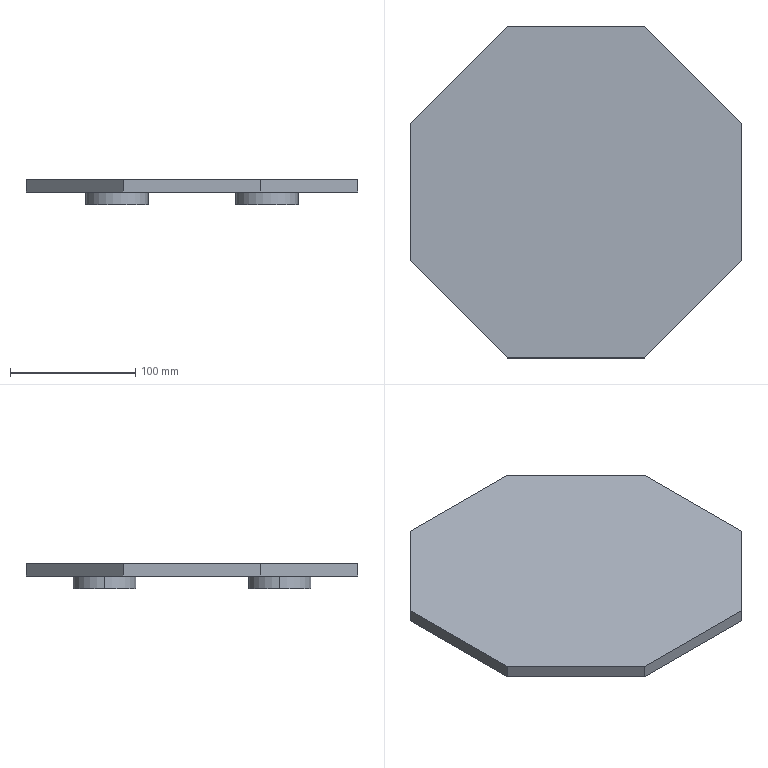Part | SolidWorks | features Extrusion 1, ICE 1 | 1 solid | 28 faces | box 265.563 x 265.563 x 20 mm | volume 605445 mm3 | plane 16 | cylinder 12 | commonest cylinder face diameters 40 x6 50 x6
STEP:
#1=CARTESIAN_POINT('',(-559.884,-160.,-10.));
#2=VERTEX_POINT('',#1);
#3=CARTESIAN_POINT('',(-519.884,-160.,-10.));
#4=VERTEX_POINT('',#3);
#5=CARTESIAN_POINT('',(-539.884,-160.,-10.));
#6=DIRECTION('',(0.,0.,1.));
#7=DIRECTION('',(1.,0.,0.));
#8=AXIS2_PLACEMENT_3D('',#5,#6,#7);
#9=CIRCLE('',#8,20.);
#10=EDGE_CURVE('',#2,#4,#9,.T.);
#11=ORIENTED_EDGE('',*,*,#10,.F.);
#12=CARTESIAN_POINT('',(-559.884,-160.,0.));
#13=VERTEX_POINT('',#12);
#14=CARTESIAN_POINT('',(-559.884,-160.,-10.));
#15=DIRECTION('',(0.,0.,1.));
#16=VECTOR('',#15,1000.);
#17=LINE('',#14,#16);
#18=EDGE_CURVE('',#2,#13,#17,.T.);
#19=ORIENTED_EDGE('',*,*,#18,.T.);
#20=CARTESIAN_POINT('',(-519.884,-160.,0.));
#21=VERTEX_POINT('',#20);
#22=CARTESIAN_POINT('',(-539.884,-160.,0.));
#23=DIRECTION('',(0.,0.,1.));
#24=DIRECTION('',(1.,0.,0.));
#25=AXIS2_PLACEMENT_3D('',#22,#23,#24);
#26=CIRCLE('',#25,20.);
#27=EDGE_CURVE('',#13,#21,#26,.T.);
#28=ORIENTED_EDGE('',*,*,#27,.T.);
#29=CARTESIAN_POINT('',(-519.884,-160.,-10.));
#30=DIRECTION('',(0.,0.,1.));
#31=VECTOR('',#30,1000.);
#32=LINE('',#29,#31);
#33=EDGE_CURVE('',#4,#21,#32,.T.);
#34=ORIENTED_EDGE('',*,*,#33,.F.);
#35=EDGE_LOOP('',(#11,#19,#28,#34));
#36=FACE_OUTER_BOUND('',#35,.T.);
#37=CARTESIAN_POINT('',(-539.884,-160.,-10.));
#38=DIRECTION('',(0.,0.,1.));
#39=DIRECTION('',(1.,0.,0.));
#40=AXIS2_PLACEMENT_3D('',#37,#38,#39);
#41=CYLINDRICAL_SURFACE('',#40,20.);
#42=ADVANCED_FACE('',(#36),#41,.F.);
#43=CARTESIAN_POINT('',(-514.884,-160.,-10.));
#44=VERTEX_POINT('',#43);
#45=CARTESIAN_POINT('',(-564.884,-160.,-10.));
#46=VERTEX_POINT('',#45);
#47=CARTESIAN_POINT('',(-539.884,-160.,-10.));
#48=DIRECTION('',(0.,0.,1.));
#49=DIRECTION('',(1.,0.,0.));
#50=AXIS2_PLACEMENT_3D('',#47,#48,#49);
#51=CIRCLE('',#50,25.);
#52=EDGE_CURVE('',#44,#46,#51,.T.);
#53=ORIENTED_EDGE('',*,*,#52,.T.);
#54=CARTESIAN_POINT('',(-564.884,-160.,0.));
#55=VERTEX_POINT('',#54);
#56=CARTESIAN_POINT('',(-564.884,-160.,-10.));
#57=DIRECTION('',(0.,0.,1.));
#58=VECTOR('',#57,1000.);
#59=LINE('',#56,#58);
#60=EDGE_CURVE('',#46,#55,#59,.T.);
#61=ORIENTED_EDGE('',*,*,#60,.T.);
#62=CARTESIAN_POINT('',(-514.884,-160.,0.));
#63=VERTEX_POINT('',#62);
#64=CARTESIAN_POINT('',(-539.884,-160.,0.));
#65=DIRECTION('',(0.,0.,1.));
#66=DIRECTION('',(1.,0.,0.));
#67=AXIS2_PLACEMENT_3D('',#64,#65,#66);
#68=CIRCLE('',#67,25.);
#69=EDGE_CURVE('',#63,#55,#68,.T.);
#70=ORIENTED_EDGE('',*,*,#69,.F.);
#71=CARTESIAN_POINT('',(-514.884,-160.,-10.));
#72=DIRECTION('',(0.,0.,1.));
#73=VECTOR('',#72,1000.);
#74=LINE('',#71,#73);
#75=EDGE_CURVE('',#44,#63,#74,.T.);
#76=ORIENTED_EDGE('',*,*,#75,.F.);
#77=EDGE_LOOP('',(#53,#61,#70,#76));
#78=FACE_OUTER_BOUND('',#77,.T.);
#79=CARTESIAN_POINT('',(-539.884,-160.,-10.));
#80=DIRECTION('',(0.,0.,1.));
#81=DIRECTION('',(1.,0.,0.));
#82=AXIS2_PLACEMENT_3D('',#79,#80,#81);
#83=CYLINDRICAL_SURFACE('',#82,25.);
#84=ADVANCED_FACE('',(#78),#83,.T.);
#85=CARTESIAN_POINT('',(-559.884,-20.,-10.));
#86=VERTEX_POINT('',#85);
#87=CARTESIAN_POINT('',(-519.884,-20.,-10.));
#88=VERTEX_POINT('',#87);
#89=CARTESIAN_POINT('',(-539.884,-20.,-10.));
#90=DIRECTION('',(0.,0.,1.));
#91=DIRECTION('',(1.,0.,0.));
#92=AXIS2_PLACEMENT_3D('',#89,#90,#91);
#93=CIRCLE('',#92,20.);
#94=EDGE_CURVE('',#86,#88,#93,.T.);
#95=ORIENTED_EDGE('',*,*,#94,.F.);
#96=CARTESIAN_POINT('',(-559.884,-20.,0.));
#97=VERTEX_POINT('',#96);
#98=CARTESIAN_POINT('',(-559.884,-20.,-10.));
#99=DIRECTION('',(0.,0.,1.));
#100=VECTOR('',#99,1000.);
#101=LINE('',#98,#100);
#102=EDGE_CURVE('',#86,#97,#101,.T.);
#103=ORIENTED_EDGE('',*,*,#102,.T.);
#104=CARTESIAN_POINT('',(-519.884,-20.,0.));
#105=VERTEX_POINT('',#104);
#106=CARTESIAN_POINT('',(-539.884,-20.,0.));
#107=DIRECTION('',(0.,0.,1.));
#108=DIRECTION('',(1.,0.,0.));
#109=AXIS2_PLACEMENT_3D('',#106,#107,#108);
#110=CIRCLE('',#109,20.);
#111=EDGE_CURVE('',#97,#105,#110,.T.);
#112=ORIENTED_EDGE('',*,*,#111,.T.);
#113=CARTESIAN_POINT('',(-519.884,-20.,-10.));
#114=DIRECTION('',(0.,0.,1.));
#115=VECTOR('',#114,1000.);
#116=LINE('',#113,#115);
#117=EDGE_CURVE('',#88,#105,#116,.T.);
#118=ORIENTED_EDGE('',*,*,#117,.F.);
#119=EDGE_LOOP('',(#95,#103,#112,#118));
#120=FACE_OUTER_BOUND('',#119,.T.);
#121=CARTESIAN_POINT('',(-539.884,-20.,-10.));
#122=DIRECTION('',(0.,0.,1.));
#123=DIRECTION('',(1.,0.,0.));
#124=AXIS2_PLACEMENT_3D('',#121,#122,#123);
#125=CYLINDRICAL_SURFACE('',#124,20.);
#126=ADVANCED_FACE('',(#120),#125,.F.);
#127=CARTESIAN_POINT('',(-514.884,-20.,-10.));
#128=VERTEX_POINT('',#127);
#129=CARTESIAN_POINT('',(-564.884,-20.,-10.));
#130=VERTEX_POINT('',#129);
#131=CARTESIAN_POINT('',(-539.884,-20.,-10.));
#132=DIRECTION('',(0.,0.,1.));
#133=DIRECTION('',(1.,0.,0.));
#134=AXIS2_PLACEMENT_3D('',#131,#132,#133);
#135=CIRCLE('',#134,25.);
#136=EDGE_CURVE('',#128,#130,#135,.T.);
#137=ORIENTED_EDGE('',*,*,#136,.T.);
#138=CARTESIAN_POINT('',(-564.884,-20.,0.));
#139=VERTEX_POINT('',#138);
#140=CARTESIAN_POINT('',(-564.884,-20.,-10.));
#141=DIRECTION('',(0.,0.,1.));
#142=VECTOR('',#141,1000.);
#143=LINE('',#140,#142);
#144=EDGE_CURVE('',#130,#139,#143,.T.);
#145=ORIENTED_EDGE('',*,*,#144,.T.);
#146=CARTESIAN_POINT('',(-514.884,-20.,0.));
#147=VERTEX_POINT('',#146);
#148=CARTESIAN_POINT('',(-539.884,-20.,0.));
#149=DIRECTION('',(0.,0.,1.));
#150=DIRECTION('',(1.,0.,0.));
#151=AXIS2_PLACEMENT_3D('',#148,#149,#150);
#152=CIRCLE('',#151,25.);
#153=EDGE_CURVE('',#147,#139,#152,.T.);
#154=ORIENTED_EDGE('',*,*,#153,.F.);
#155=CARTESIAN_POINT('',(-514.884,-20.,-10.));
#156=DIRECTION('',(0.,0.,1.));
#157=VECTOR('',#156,1000.);
#158=LINE('',#155,#157);
#159=EDGE_CURVE('',#128,#147,#158,.T.);
#160=ORIENTED_EDGE('',*,*,#159,.F.);
#161=EDGE_LOOP('',(#137,#145,#154,#160));
#162=FACE_OUTER_BOUND('',#161,.T.);
#163=CARTESIAN_POINT('',(-539.884,-20.,-10.));
#164=DIRECTION('',(0.,0.,1.));
#165=DIRECTION('',(1.,0.,0.));
#166=AXIS2_PLACEMENT_3D('',#163,#164,#165);
#167=CYLINDRICAL_SURFACE('',#166,25.);
#168=ADVANCED_FACE('',(#162),#167,.T.);
#169=CARTESIAN_POINT('',(-679.884,-20.,-10.));
#170=VERTEX_POINT('',#169);
#171=CARTESIAN_POINT('',(-639.884,-20.,-10.));
#172=VERTEX_POINT('',#171);
#173=CARTESIAN_POINT('',(-659.884,-20.,-10.));
#174=DIRECTION('',(0.,0.,1.));
#175=DIRECTION('',(1.,0.,0.));
#176=AXIS2_PLACEMENT_3D('',#173,#174,#175);
#177=CIRCLE('',#176,20.);
#178=EDGE_CURVE('',#170,#172,#177,.T.);
#179=ORIENTED_EDGE('',*,*,#178,.F.);
#180=CARTESIAN_POINT('',(-679.884,-20.,0.));
#181=VERTEX_POINT('',#180);
#182=CARTESIAN_POINT('',(-679.884,-20.,-10.));
#183=DIRECTION('',(0.,0.,1.));
#184=VECTOR('',#183,1000.);
#185=LINE('',#182,#184);
#186=EDGE_CURVE('',#170,#181,#185,.T.);
#187=ORIENTED_EDGE('',*,*,#186,.T.);
#188=CARTESIAN_POINT('',(-639.884,-20.,0.));
#189=VERTEX_POINT('',#188);
#190=CARTESIAN_POINT('',(-659.884,-20.,0.));
#191=DIRECTION('',(0.,0.,1.));
#192=DIRECTION('',(1.,0.,0.));
#193=AXIS2_PLACEMENT_3D('',#190,#191,#192);
#194=CIRCLE('',#193,20.);
#195=EDGE_CURVE('',#181,#189,#194,.T.);
#196=ORIENTED_EDGE('',*,*,#195,.T.);
#197=CARTESIAN_POINT('',(-639.884,-20.,-10.));
#198=DIRECTION('',(0.,0.,1.));
#199=VECTOR('',#198,1000.);
#200=LINE('',#197,#199);
#201=EDGE_CURVE('',#172,#189,#200,.T.);
#202=ORIENTED_EDGE('',*,*,#201,.F.);
#203=EDGE_LOOP('',(#179,#187,#196,#202));
#204=FACE_OUTER_BOUND('',#203,.T.);
#205=CARTESIAN_POINT('',(-659.884,-20.,-10.));
#206=DIRECTION('',(0.,0.,1.));
#207=DIRECTION('',(1.,0.,0.));
#208=AXIS2_PLACEMENT_3D('',#205,#206,#207);
#209=CYLINDRICAL_SURFACE('',#208,20.);
#210=ADVANCED_FACE('',(#204),#209,.F.);
#211=CARTESIAN_POINT('',(-634.884,-20.,-10.));
#212=VERTEX_POINT('',#211);
#213=CARTESIAN_POINT('',(-684.884,-20.,-10.));
#214=VERTEX_POINT('',#213);
#215=CARTESIAN_POINT('',(-659.884,-20.,-10.));
#216=DIRECTION('',(0.,0.,1.));
#217=DIRECTION('',(1.,0.,0.));
#218=AXIS2_PLACEMENT_3D('',#215,#216,#217);
#219=CIRCLE('',#218,25.);
#220=EDGE_CURVE('',#212,#214,#219,.T.);
#221=ORIENTED_EDGE('',*,*,#220,.T.);
#222=CARTESIAN_POINT('',(-684.884,-20.,0.));
#223=VERTEX_POINT('',#222);
#224=CARTESIAN_POINT('',(-684.884,-20.,-10.));
#225=DIRECTION('',(0.,0.,1.));
#226=VECTOR('',#225,1000.);
#227=LINE('',#224,#226);
#228=EDGE_CURVE('',#214,#223,#227,.T.);
#229=ORIENTED_EDGE('',*,*,#228,.T.);
#230=CARTESIAN_POINT('',(-634.884,-20.,0.));
#231=VERTEX_POINT('',#230);
#232=CARTESIAN_POINT('',(-659.884,-20.,0.));
#233=DIRECTION('',(0.,0.,1.));
#234=DIRECTION('',(1.,0.,0.));
#235=AXIS2_PLACEMENT_3D('',#232,#233,#234);
#236=CIRCLE('',#235,25.);
#237=EDGE_CURVE('',#231,#223,#236,.T.);
#238=ORIENTED_EDGE('',*,*,#237,.F.);
#239=CARTESIAN_POINT('',(-634.884,-20.,-10.));
#240=DIRECTION('',(0.,0.,1.));
#241=VECTOR('',#240,1000.);
#242=LINE('',#239,#241);
#243=EDGE_CURVE('',#212,#231,#242,.T.);
#244=ORIENTED_EDGE('',*,*,#243,.F.);
#245=EDGE_LOOP('',(#221,#229,#238,#244));
#246=FACE_OUTER_BOUND('',#245,.T.);
#247=CARTESIAN_POINT('',(-659.884,-20.,-10.));
#248=DIRECTION('',(0.,0.,1.));
#249=DIRECTION('',(1.,0.,0.));
#250=AXIS2_PLACEMENT_3D('',#247,#248,#249);
#251=CYLINDRICAL_SURFACE('',#250,25.);
#252=ADVANCED_FACE('',(#246),#251,.T.);
#253=ORIENTED_EDGE('',*,*,#228,.F.);
#254=CARTESIAN_POINT('',(-659.884,-20.,-10.));
#255=DIRECTION('',(0.,0.,1.));
#256=DIRECTION('',(1.,0.,0.));
#257=AXIS2_PLACEMENT_3D('',#254,#255,#256);
#258=CIRCLE('',#257,25.);
#259=EDGE_CURVE('',#214,#212,#258,.T.);
#260=ORIENTED_EDGE('',*,*,#259,.T.);
#261=ORIENTED_EDGE('',*,*,#243,.T.);
#262=CARTESIAN_POINT('',(-659.884,-20.,0.));
#263=DIRECTION('',(0.,0.,1.));
#264=DIRECTION('',(1.,0.,0.));
#265=AXIS2_PLACEMENT_3D('',#262,#263,#264);
#266=CIRCLE('',#265,25.);
#267=EDGE_CURVE('',#223,#231,#266,.T.);
#268=ORIENTED_EDGE('',*,*,#267,.F.);
#269=EDGE_LOOP('',(#253,#260,#261,#268));
#270=FACE_OUTER_BOUND('',#269,.T.);
#271=CARTESIAN_POINT('',(-659.884,-20.,-10.));
#272=DIRECTION('',(0.,0.,1.));
#273=DIRECTION('',(1.,0.,0.));
#274=AXIS2_PLACEMENT_3D('',#271,#272,#273);
#275=CYLINDRICAL_SURFACE('',#274,25.);
#276=ADVANCED_FACE('',(#270),#275,.T.);
#277=CARTESIAN_POINT('',(-659.884,-20.,-10.));
#278=DIRECTION('',(0.,0.,1.));
#279=DIRECTION('',(1.,0.,0.));
#280=AXIS2_PLACEMENT_3D('',#277,#278,#279);
#281=CIRCLE('',#280,20.);
#282=EDGE_CURVE('',#172,#170,#281,.T.);
#283=ORIENTED_EDGE('',*,*,#282,.T.);
#284=ORIENTED_EDGE('',*,*,#178,.T.);
#285=EDGE_LOOP('',(#283,#284));
#286=FACE_BOUND('',#285,.T.);
#287=ORIENTED_EDGE('',*,*,#220,.F.);
#288=ORIENTED_EDGE('',*,*,#259,.F.);
#289=EDGE_LOOP('',(#287,#288));
#290=FACE_OUTER_BOUND('',#289,.T.);
#291=CARTESIAN_POINT('',(-659.884,-20.,-10.));
#292=DIRECTION('',(0.,0.,1.));
#293=DIRECTION('',(1.,0.,0.));
#294=AXIS2_PLACEMENT_3D('',#291,#292,#293);
#295=PLANE('',#294);
#296=ADVANCED_FACE('',(#286,#290),#295,.F.);
#297=ORIENTED_EDGE('',*,*,#186,.F.);
#298=ORIENTED_EDGE('',*,*,#282,.F.);
#299=ORIENTED_EDGE('',*,*,#201,.T.);
#300=CARTESIAN_POINT('',(-659.884,-20.,0.));
#301=DIRECTION('',(0.,0.,1.));
#302=DIRECTION('',(1.,0.,0.));
#303=AXIS2_PLACEMENT_3D('',#300,#301,#302);
#304=CIRCLE('',#303,20.);
#305=EDGE_CURVE('',#189,#181,#304,.T.);
#306=ORIENTED_EDGE('',*,*,#305,.T.);
#307=EDGE_LOOP('',(#297,#298,#299,#306));
#308=FACE_OUTER_BOUND('',#307,.T.);
#309=CARTESIAN_POINT('',(-659.884,-20.,-10.));
#310=DIRECTION('',(0.,0.,1.));
#311=DIRECTION('',(1.,0.,0.));
#312=AXIS2_PLACEMENT_3D('',#309,#310,#311);
#313=CYLINDRICAL_SURFACE('',#312,20.);
#314=ADVANCED_FACE('',(#308),#313,.F.);
#315=ORIENTED_EDGE('',*,*,#69,.T.);
#316=CARTESIAN_POINT('',(-539.884,-160.,0.));
#317=DIRECTION('',(0.,0.,1.));
#318=DIRECTION('',(1.,0.,0.));
#319=AXIS2_PLACEMENT_3D('',#316,#317,#318);
#320=CIRCLE('',#319,25.);
#321=EDGE_CURVE('',#55,#63,#320,.T.);
#322=ORIENTED_EDGE('',*,*,#321,.T.);
#323=EDGE_LOOP('',(#315,#322));
#324=FACE_BOUND('',#323,.T.);
#325=ORIENTED_EDGE('',*,*,#153,.T.);
#326=CARTESIAN_POINT('',(-539.884,-20.,0.));
#327=DIRECTION('',(0.,0.,1.));
#328=DIRECTION('',(1.,0.,0.));
#329=AXIS2_PLACEMENT_3D('',#326,#327,#328);
#330=CIRCLE('',#329,25.);
#331=EDGE_CURVE('',#139,#147,#330,.T.);
#332=ORIENTED_EDGE('',*,*,#331,.T.);
#333=EDGE_LOOP('',(#325,#332));
#334=FACE_BOUND('',#333,.T.);
#335=ORIENTED_EDGE('',*,*,#237,.T.);
#336=ORIENTED_EDGE('',*,*,#267,.T.);
#337=EDGE_LOOP('',(#335,#336));
#338=FACE_BOUND('',#337,.T.);
#339=CARTESIAN_POINT('',(-654.884,-222.782,0.));
#340=VERTEX_POINT('',#339);
#341=CARTESIAN_POINT('',(-544.884,-222.782,0.));
#342=VERTEX_POINT('',#341);
#343=CARTESIAN_POINT('',(-654.884,-222.782,0.));
#344=DIRECTION('',(1.,0.,0.));
#345=VECTOR('',#344,1000.);
#346=LINE('',#343,#345);
#347=EDGE_CURVE('',#340,#342,#346,.T.);
#348=ORIENTED_EDGE('',*,*,#347,.F.);
#349=CARTESIAN_POINT('',(-732.666,-145.,0.));
#350=VERTEX_POINT('',#349);
#351=CARTESIAN_POINT('',(-732.666,-145.,0.));
#352=DIRECTION('',(0.7071,-0.7071,0.));
#353=VECTOR('',#352,1000.);
#354=LINE('',#351,#353);
#355=EDGE_CURVE('',#350,#340,#354,.T.);
#356=ORIENTED_EDGE('',*,*,#355,.F.);
#357=CARTESIAN_POINT('',(-732.666,-35.,0.));
#358=VERTEX_POINT('',#357);
#359=CARTESIAN_POINT('',(-732.666,-35.,0.));
#360=DIRECTION('',(0.,-1.,0.));
#361=VECTOR('',#360,1000.);
#362=LINE('',#359,#361);
#363=EDGE_CURVE('',#358,#350,#362,.T.);
#364=ORIENTED_EDGE('',*,*,#363,.F.);
#365=CARTESIAN_POINT('',(-654.884,42.782,0.));
#366=VERTEX_POINT('',#365);
#367=CARTESIAN_POINT('',(-654.884,42.782,0.));
#368=DIRECTION('',(-0.7071,-0.7071,0.));
#369=VECTOR('',#368,1000.);
#370=LINE('',#367,#369);
#371=EDGE_CURVE('',#366,#358,#370,.T.);
#372=ORIENTED_EDGE('',*,*,#371,.F.);
#373=CARTESIAN_POINT('',(-544.884,42.782,0.));
#374=VERTEX_POINT('',#373);
#375=CARTESIAN_POINT('',(-544.884,42.782,0.));
#376=DIRECTION('',(-1.,0.,0.));
#377=VECTOR('',#376,1000.);
#378=LINE('',#375,#377);
#379=EDGE_CURVE('',#374,#366,#378,.T.);
#380=ORIENTED_EDGE('',*,*,#379,.F.);
#381=CARTESIAN_POINT('',(-467.102,-35.,0.));
#382=VERTEX_POINT('',#381);
#383=CARTESIAN_POINT('',(-467.102,-35.,0.));
#384=DIRECTION('',(-0.7071,0.7071,0.));
#385=VECTOR('',#384,1000.);
#386=LINE('',#383,#385);
#387=EDGE_CURVE('',#382,#374,#386,.T.);
#388=ORIENTED_EDGE('',*,*,#387,.F.);
#389=CARTESIAN_POINT('',(-467.102,-145.,0.));
#390=VERTEX_POINT('',#389);
#391=CARTESIAN_POINT('',(-467.102,-145.,0.));
#392=DIRECTION('',(0.,1.,0.));
#393=VECTOR('',#392,1000.);
#394=LINE('',#391,#393);
#395=EDGE_CURVE('',#390,#382,#394,.T.);
#396=ORIENTED_EDGE('',*,*,#395,.F.);
#397=CARTESIAN_POINT('',(-544.884,-222.782,0.));
#398=DIRECTION('',(0.7071,0.7071,0.));
#399=VECTOR('',#398,1000.);
#400=LINE('',#397,#399);
#401=EDGE_CURVE('',#342,#390,#400,.T.);
#402=ORIENTED_EDGE('',*,*,#401,.F.);
#403=EDGE_LOOP('',(#348,#356,#364,#372,#380,#388,#396,#402));
#404=FACE_OUTER_BOUND('',#403,.T.);
#405=CARTESIAN_POINT('',(0.,0.,0.));
#406=DIRECTION('',(0.,0.,1.));
#407=DIRECTION('',(1.,0.,0.));
#408=AXIS2_PLACEMENT_3D('',#405,#406,#407);
#409=PLANE('',#408);
#410=ADVANCED_FACE('',(#324,#334,#338,#404),#409,.F.);
#411=CARTESIAN_POINT('',(-654.884,-222.782,10.));
#412=VERTEX_POINT('',#411);
#413=CARTESIAN_POINT('',(-544.884,-222.782,10.));
#414=VERTEX_POINT('',#413);
#415=CARTESIAN_POINT('',(-654.884,-222.782,10.));
#416=DIRECTION('',(1.,0.,0.));
#417=VECTOR('',#416,1000.);
#418=LINE('',#415,#417);
#419=EDGE_CURVE('',#412,#414,#418,.T.);
#420=ORIENTED_EDGE('',*,*,#419,.T.);
#421=CARTESIAN_POINT('',(-467.102,-145.,10.));
#422=VERTEX_POINT('',#421);
#423=CARTESIAN_POINT('',(-544.884,-222.782,10.));
#424=DIRECTION('',(0.7071,0.7071,0.));
#425=VECTOR('',#424,1000.);
#426=LINE('',#423,#425);
#427=EDGE_CURVE('',#414,#422,#426,.T.);
#428=ORIENTED_EDGE('',*,*,#427,.T.);
#429=CARTESIAN_POINT('',(-467.102,-35.,10.));
#430=VERTEX_POINT('',#429);
#431=CARTESIAN_POINT('',(-467.102,-145.,10.));
#432=DIRECTION('',(0.,1.,0.));
#433=VECTOR('',#432,1000.);
#434=LINE('',#431,#433);
#435=EDGE_CURVE('',#422,#430,#434,.T.);
#436=ORIENTED_EDGE('',*,*,#435,.T.);
#437=CARTESIAN_POINT('',(-544.884,42.782,10.));
#438=VERTEX_POINT('',#437);
#439=CARTESIAN_POINT('',(-467.102,-35.,10.));
#440=DIRECTION('',(-0.7071,0.7071,0.));
#441=VECTOR('',#440,1000.);
#442=LINE('',#439,#441);
#443=EDGE_CURVE('',#430,#438,#442,.T.);
#444=ORIENTED_EDGE('',*,*,#443,.T.);
#445=CARTESIAN_POINT('',(-654.884,42.782,10.));
#446=VERTEX_POINT('',#445);
#447=CARTESIAN_POINT('',(-544.884,42.782,10.));
#448=DIRECTION('',(-1.,0.,0.));
#449=VECTOR('',#448,1000.);
#450=LINE('',#447,#449);
#451=EDGE_CURVE('',#438,#446,#450,.T.);
#452=ORIENTED_EDGE('',*,*,#451,.T.);
#453=CARTESIAN_POINT('',(-732.666,-35.,10.));
#454=VERTEX_POINT('',#453);
#455=CARTESIAN_POINT('',(-654.884,42.782,10.));
#456=DIRECTION('',(-0.7071,-0.7071,0.));
#457=VECTOR('',#456,1000.);
#458=LINE('',#455,#457);
#459=EDGE_CURVE('',#446,#454,#458,.T.);
#460=ORIENTED_EDGE('',*,*,#459,.T.);
#461=CARTESIAN_POINT('',(-732.666,-145.,10.));
#462=VERTEX_POINT('',#461);
#463=CARTESIAN_POINT('',(-732.666,-35.,10.));
#464=DIRECTION('',(0.,-1.,0.));
#465=VECTOR('',#464,1000.);
#466=LINE('',#463,#465);
#467=EDGE_CURVE('',#454,#462,#466,.T.);
#468=ORIENTED_EDGE('',*,*,#467,.T.);
#469=CARTESIAN_POINT('',(-732.666,-145.,10.));
#470=DIRECTION('',(0.7071,-0.7071,0.));
#471=VECTOR('',#470,1000.);
#472=LINE('',#469,#471);
#473=EDGE_CURVE('',#462,#412,#472,.T.);
#474=ORIENTED_EDGE('',*,*,#473,.T.);
#475=EDGE_LOOP('',(#420,#428,#436,#444,#452,#460,#468,#474));
#476=FACE_OUTER_BOUND('',#475,.T.);
#477=CARTESIAN_POINT('',(0.,0.,10.));
#478=DIRECTION('',(0.,0.,1.));
#479=DIRECTION('',(1.,0.,0.));
#480=AXIS2_PLACEMENT_3D('',#477,#478,#479);
#481=PLANE('',#480);
#482=ADVANCED_FACE('',(#476),#481,.T.);
#483=ORIENTED_EDGE('',*,*,#355,.T.);
#484=CARTESIAN_POINT('',(-654.884,-222.782,10.));
#485=DIRECTION('',(0.,0.,-1.));
#486=VECTOR('',#485,1000.);
#487=LINE('',#484,#486);
#488=EDGE_CURVE('',#412,#340,#487,.T.);
#489=ORIENTED_EDGE('',*,*,#488,.F.);
#490=ORIENTED_EDGE('',*,*,#473,.F.);
#491=CARTESIAN_POINT('',(-732.666,-145.,10.));
#492=DIRECTION('',(0.,0.,-1.));
#493=VECTOR('',#492,1000.);
#494=LINE('',#491,#493);
#495=EDGE_CURVE('',#462,#350,#494,.T.);
#496=ORIENTED_EDGE('',*,*,#495,.T.);
#497=EDGE_LOOP('',(#483,#489,#490,#496));
#498=FACE_OUTER_BOUND('',#497,.T.);
#499=CARTESIAN_POINT('',(-732.666,-145.,10.));
#500=DIRECTION('',(0.7071,0.7071,0.));
#501=DIRECTION('',(-0.7071,0.7071,0.));
#502=AXIS2_PLACEMENT_3D('',#499,#500,#501);
#503=PLANE('',#502);
#504=ADVANCED_FACE('',(#498),#503,.F.);
#505=ORIENTED_EDGE('',*,*,#363,.T.);
#506=ORIENTED_EDGE('',*,*,#495,.F.);
#507=ORIENTED_EDGE('',*,*,#467,.F.);
#508=CARTESIAN_POINT('',(-732.666,-35.,10.));
#509=DIRECTION('',(0.,0.,-1.));
#510=VECTOR('',#509,1000.);
#511=LINE('',#508,#510);
#512=EDGE_CURVE('',#454,#358,#511,.T.);
#513=ORIENTED_EDGE('',*,*,#512,.T.);
#514=EDGE_LOOP('',(#505,#506,#507,#513));
#515=FACE_OUTER_BOUND('',#514,.T.);
#516=CARTESIAN_POINT('',(-732.666,-35.,10.));
#517=DIRECTION('',(1.,0.,0.));
#518=DIRECTION('',(0.,0.,-1.));
#519=AXIS2_PLACEMENT_3D('',#516,#517,#518);
#520=PLANE('',#519);
#521=ADVANCED_FACE('',(#515),#520,.F.);
#522=ORIENTED_EDGE('',*,*,#371,.T.);
#523=ORIENTED_EDGE('',*,*,#512,.F.);
#524=ORIENTED_EDGE('',*,*,#459,.F.);
#525=CARTESIAN_POINT('',(-654.884,42.782,10.));
#526=DIRECTION('',(0.,0.,-1.));
#527=VECTOR('',#526,1000.);
#528=LINE('',#525,#527);
#529=EDGE_CURVE('',#446,#366,#528,.T.);
#530=ORIENTED_EDGE('',*,*,#529,.T.);
#531=EDGE_LOOP('',(#522,#523,#524,#530));
#532=FACE_OUTER_BOUND('',#531,.T.);
#533=CARTESIAN_POINT('',(-654.884,42.782,10.));
#534=DIRECTION('',(0.7071,-0.7071,0.));
#535=DIRECTION('',(0.7071,0.7071,0.));
#536=AXIS2_PLACEMENT_3D('',#533,#534,#535);
#537=PLANE('',#536);
#538=ADVANCED_FACE('',(#532),#537,.F.);
#539=ORIENTED_EDGE('',*,*,#379,.T.);
#540=ORIENTED_EDGE('',*,*,#529,.F.);
#541=ORIENTED_EDGE('',*,*,#451,.F.);
#542=CARTESIAN_POINT('',(-544.884,42.782,10.));
#543=DIRECTION('',(0.,0.,-1.));
#544=VECTOR('',#543,1000.);
#545=LINE('',#542,#544);
#546=EDGE_CURVE('',#438,#374,#545,.T.);
#547=ORIENTED_EDGE('',*,*,#546,.T.);
#548=EDGE_LOOP('',(#539,#540,#541,#547));
#549=FACE_OUTER_BOUND('',#548,.T.);
#550=CARTESIAN_POINT('',(-544.884,42.782,10.));
#551=DIRECTION('',(0.,-1.,0.));
#552=DIRECTION('',(1.,0.,0.));
#553=AXIS2_PLACEMENT_3D('',#550,#551,#552);
#554=PLANE('',#553);
#555=ADVANCED_FACE('',(#549),#554,.F.);
#556=ORIENTED_EDGE('',*,*,#387,.T.);
#557=ORIENTED_EDGE('',*,*,#546,.F.);
#558=ORIENTED_EDGE('',*,*,#443,.F.);
#559=CARTESIAN_POINT('',(-467.102,-35.,10.));
#560=DIRECTION('',(0.,0.,-1.));
#561=VECTOR('',#560,1000.);
#562=LINE('',#559,#561);
#563=EDGE_CURVE('',#430,#382,#562,.T.);
#564=ORIENTED_EDGE('',*,*,#563,.T.);
#565=EDGE_LOOP('',(#556,#557,#558,#564));
#566=FACE_OUTER_BOUND('',#565,.T.);
#567=CARTESIAN_POINT('',(-467.102,-35.,10.));
#568=DIRECTION('',(-0.7071,-0.7071,0.));
#569=DIRECTION('',(0.7071,-0.7071,0.));
#570=AXIS2_PLACEMENT_3D('',#567,#568,#569);
#571=PLANE('',#570);
#572=ADVANCED_FACE('',(#566),#571,.F.);
#573=ORIENTED_EDGE('',*,*,#395,.T.);
#574=ORIENTED_EDGE('',*,*,#563,.F.);
#575=ORIENTED_EDGE('',*,*,#435,.F.);
#576=CARTESIAN_POINT('',(-467.102,-145.,10.));
#577=DIRECTION('',(0.,0.,-1.));
#578=VECTOR('',#577,1000.);
#579=LINE('',#576,#578);
#580=EDGE_CURVE('',#422,#390,#579,.T.);
#581=ORIENTED_EDGE('',*,*,#580,.T.);
#582=EDGE_LOOP('',(#573,#574,#575,#581));
#583=FACE_OUTER_BOUND('',#582,.T.);
#584=CARTESIAN_POINT('',(-467.102,-145.,10.));
#585=DIRECTION('',(-1.,0.,0.));
#586=DIRECTION('',(0.,0.,1.));
#587=AXIS2_PLACEMENT_3D('',#584,#585,#586);
#588=PLANE('',#587);
#589=ADVANCED_FACE('',(#583),#588,.F.);
#590=ORIENTED_EDGE('',*,*,#401,.T.);
#591=ORIENTED_EDGE('',*,*,#580,.F.);
#592=ORIENTED_EDGE('',*,*,#427,.F.);
#593=CARTESIAN_POINT('',(-544.884,-222.782,10.));
#594=DIRECTION('',(0.,0.,-1.));
#595=VECTOR('',#594,1000.);
#596=LINE('',#593,#595);
#597=EDGE_CURVE('',#414,#342,#596,.T.);
#598=ORIENTED_EDGE('',*,*,#597,.T.);
#599=EDGE_LOOP('',(#590,#591,#592,#598));
#600=FACE_OUTER_BOUND('',#599,.T.);
#601=CARTESIAN_POINT('',(-544.884,-222.782,10.));
#602=DIRECTION('',(-0.7071,0.7071,0.));
#603=DIRECTION('',(-0.7071,-0.7071,0.));
#604=AXIS2_PLACEMENT_3D('',#601,#602,#603);
#605=PLANE('',#604);
#606=ADVANCED_FACE('',(#600),#605,.F.);
#607=ORIENTED_EDGE('',*,*,#347,.T.);
#608=ORIENTED_EDGE('',*,*,#597,.F.);
#609=ORIENTED_EDGE('',*,*,#419,.F.);
#610=ORIENTED_EDGE('',*,*,#488,.T.);
#611=EDGE_LOOP('',(#607,#608,#609,#610));
#612=FACE_OUTER_BOUND('',#611,.T.);
#613=CARTESIAN_POINT('',(-654.884,-222.782,10.));
#614=DIRECTION('',(0.,1.,0.));
#615=DIRECTION('',(0.,0.,1.));
#616=AXIS2_PLACEMENT_3D('',#613,#614,#615);
#617=PLANE('',#616);
#618=ADVANCED_FACE('',(#612),#617,.F.);
#619=ORIENTED_EDGE('',*,*,#305,.F.);
#620=ORIENTED_EDGE('',*,*,#195,.F.);
#621=EDGE_LOOP('',(#619,#620));
#622=FACE_OUTER_BOUND('',#621,.T.);
#623=CARTESIAN_POINT('',(0.,0.,0.));
#624=DIRECTION('',(0.,0.,1.));
#625=DIRECTION('',(1.,0.,0.));
#626=AXIS2_PLACEMENT_3D('',#623,#624,#625);
#627=PLANE('',#626);
#628=ADVANCED_FACE('',(#622),#627,.F.);
#629=ORIENTED_EDGE('',*,*,#144,.F.);
#630=CARTESIAN_POINT('',(-539.884,-20.,-10.));
#631=DIRECTION('',(0.,0.,1.));
#632=DIRECTION('',(1.,0.,0.));
#633=AXIS2_PLACEMENT_3D('',#630,#631,#632);
#634=CIRCLE('',#633,25.);
#635=EDGE_CURVE('',#130,#128,#634,.T.);
#636=ORIENTED_EDGE('',*,*,#635,.T.);
#637=ORIENTED_EDGE('',*,*,#159,.T.);
#638=ORIENTED_EDGE('',*,*,#331,.F.);
#639=EDGE_LOOP('',(#629,#636,#637,#638));
#640=FACE_OUTER_BOUND('',#639,.T.);
#641=CARTESIAN_POINT('',(-539.884,-20.,-10.));
#642=DIRECTION('',(0.,0.,1.));
#643=DIRECTION('',(1.,0.,0.));
#644=AXIS2_PLACEMENT_3D('',#641,#642,#643);
#645=CYLINDRICAL_SURFACE('',#644,25.);
#646=ADVANCED_FACE('',(#640),#645,.T.);
#647=CARTESIAN_POINT('',(-539.884,-20.,-10.));
#648=DIRECTION('',(0.,0.,1.));
#649=DIRECTION('',(1.,0.,0.));
#650=AXIS2_PLACEMENT_3D('',#647,#648,#649);
#651=CIRCLE('',#650,20.);
#652=EDGE_CURVE('',#88,#86,#651,.T.);
#653=ORIENTED_EDGE('',*,*,#652,.T.);
#654=ORIENTED_EDGE('',*,*,#94,.T.);
#655=EDGE_LOOP('',(#653,#654));
#656=FACE_BOUND('',#655,.T.);
#657=ORIENTED_EDGE('',*,*,#136,.F.);
#658=ORIENTED_EDGE('',*,*,#635,.F.);
#659=EDGE_LOOP('',(#657,#658));
#660=FACE_OUTER_BOUND('',#659,.T.);
#661=CARTESIAN_POINT('',(-539.884,-20.,-10.));
#662=DIRECTION('',(0.,0.,1.));
#663=DIRECTION('',(1.,0.,0.));
#664=AXIS2_PLACEMENT_3D('',#661,#662,#663);
#665=PLANE('',#664);
#666=ADVANCED_FACE('',(#656,#660),#665,.F.);
#667=ORIENTED_EDGE('',*,*,#102,.F.);
#668=ORIENTED_EDGE('',*,*,#652,.F.);
#669=ORIENTED_EDGE('',*,*,#117,.T.);
#670=CARTESIAN_POINT('',(-539.884,-20.,0.));
#671=DIRECTION('',(0.,0.,1.));
#672=DIRECTION('',(1.,0.,0.));
#673=AXIS2_PLACEMENT_3D('',#670,#671,#672);
#674=CIRCLE('',#673,20.);
#675=EDGE_CURVE('',#105,#97,#674,.T.);
#676=ORIENTED_EDGE('',*,*,#675,.T.);
#677=EDGE_LOOP('',(#667,#668,#669,#676));
#678=FACE_OUTER_BOUND('',#677,.T.);
#679=CARTESIAN_POINT('',(-539.884,-20.,-10.));
#680=DIRECTION('',(0.,0.,1.));
#681=DIRECTION('',(1.,0.,0.));
#682=AXIS2_PLACEMENT_3D('',#679,#680,#681);
#683=CYLINDRICAL_SURFACE('',#682,20.);
#684=ADVANCED_FACE('',(#678),#683,.F.);
#685=ORIENTED_EDGE('',*,*,#675,.F.);
#686=ORIENTED_EDGE('',*,*,#111,.F.);
#687=EDGE_LOOP('',(#685,#686));
#688=FACE_OUTER_BOUND('',#687,.T.);
#689=CARTESIAN_POINT('',(0.,0.,0.));
#690=DIRECTION('',(0.,0.,1.));
#691=DIRECTION('',(1.,0.,0.));
#692=AXIS2_PLACEMENT_3D('',#689,#690,#691);
#693=PLANE('',#692);
#694=ADVANCED_FACE('',(#688),#693,.F.);
#695=ORIENTED_EDGE('',*,*,#60,.F.);
#696=CARTESIAN_POINT('',(-539.884,-160.,-10.));
#697=DIRECTION('',(0.,0.,1.));
#698=DIRECTION('',(1.,0.,0.));
#699=AXIS2_PLACEMENT_3D('',#696,#697,#698);
#700=CIRCLE('',#699,25.);
#701=EDGE_CURVE('',#46,#44,#700,.T.);
#702=ORIENTED_EDGE('',*,*,#701,.T.);
#703=ORIENTED_EDGE('',*,*,#75,.T.);
#704=ORIENTED_EDGE('',*,*,#321,.F.);
#705=EDGE_LOOP('',(#695,#702,#703,#704));
#706=FACE_OUTER_BOUND('',#705,.T.);
#707=CARTESIAN_POINT('',(-539.884,-160.,-10.));
#708=DIRECTION('',(0.,0.,1.));
#709=DIRECTION('',(1.,0.,0.));
#710=AXIS2_PLACEMENT_3D('',#707,#708,#709);
#711=CYLINDRICAL_SURFACE('',#710,25.);
#712=ADVANCED_FACE('',(#706),#711,.T.);
#713=CARTESIAN_POINT('',(-539.884,-160.,-10.));
#714=DIRECTION('',(0.,0.,1.));
#715=DIRECTION('',(1.,0.,0.));
#716=AXIS2_PLACEMENT_3D('',#713,#714,#715);
#717=CIRCLE('',#716,20.);
#718=EDGE_CURVE('',#4,#2,#717,.T.);
#719=ORIENTED_EDGE('',*,*,#718,.T.);
#720=ORIENTED_EDGE('',*,*,#10,.T.);
#721=EDGE_LOOP('',(#719,#720));
#722=FACE_BOUND('',#721,.T.);
#723=ORIENTED_EDGE('',*,*,#52,.F.);
#724=ORIENTED_EDGE('',*,*,#701,.F.);
#725=EDGE_LOOP('',(#723,#724));
#726=FACE_OUTER_BOUND('',#725,.T.);
#727=CARTESIAN_POINT('',(-539.884,-160.,-10.));
#728=DIRECTION('',(0.,0.,1.));
#729=DIRECTION('',(1.,0.,0.));
#730=AXIS2_PLACEMENT_3D('',#727,#728,#729);
#731=PLANE('',#730);
#732=ADVANCED_FACE('',(#722,#726),#731,.F.);
#733=ORIENTED_EDGE('',*,*,#18,.F.);
#734=ORIENTED_EDGE('',*,*,#718,.F.);
#735=ORIENTED_EDGE('',*,*,#33,.T.);
#736=CARTESIAN_POINT('',(-539.884,-160.,0.));
#737=DIRECTION('',(0.,0.,1.));
#738=DIRECTION('',(1.,0.,0.));
#739=AXIS2_PLACEMENT_3D('',#736,#737,#738);
#740=CIRCLE('',#739,20.);
#741=EDGE_CURVE('',#21,#13,#740,.T.);
#742=ORIENTED_EDGE('',*,*,#741,.T.);
#743=EDGE_LOOP('',(#733,#734,#735,#742));
#744=FACE_OUTER_BOUND('',#743,.T.);
#745=CARTESIAN_POINT('',(-539.884,-160.,-10.));
#746=DIRECTION('',(0.,0.,1.));
#747=DIRECTION('',(1.,0.,0.));
#748=AXIS2_PLACEMENT_3D('',#745,#746,#747);
#749=CYLINDRICAL_SURFACE('',#748,20.);
#750=ADVANCED_FACE('',(#744),#749,.F.);
#751=ORIENTED_EDGE('',*,*,#741,.F.);
#752=ORIENTED_EDGE('',*,*,#27,.F.);
#753=EDGE_LOOP('',(#751,#752));
#754=FACE_OUTER_BOUND('',#753,.T.);
#755=CARTESIAN_POINT('',(0.,0.,0.));
#756=DIRECTION('',(0.,0.,1.));
#757=DIRECTION('',(1.,0.,0.));
#758=AXIS2_PLACEMENT_3D('',#755,#756,#757);
#759=PLANE('',#758);
#760=ADVANCED_FACE('',(#754),#759,.F.);
#761=CLOSED_SHELL('',(#42,#84,#126,#168,#210,#252,#276,#296,#314,#410,#482,#504,#521,#538,#555,#572,#589,#606,#618,#628,#646,#666,#684,#694,#712,#732,#750,#760));
#762=MANIFOLD_SOLID_BREP('',#761);
#763=CARTESIAN_POINT('',(0.,0.,0.));
#764=DIRECTION('',(0.,0.,1.));
#765=DIRECTION('',(1.,0.,0.));
#766=AXIS2_PLACEMENT_3D('',#763,#764,#765);
#767=(LENGTH_UNIT()NAMED_UNIT(*)SI_UNIT(.MILLI.,.METRE.));
#768=UNCERTAINTY_MEASURE_WITH_UNIT(LENGTH_MEASURE(0.00001),#767,'','');
#769=(NAMED_UNIT(*)PLANE_ANGLE_UNIT()SI_UNIT($,.RADIAN.));
#770=(NAMED_UNIT(*)SI_UNIT($,.STERADIAN.)SOLID_ANGLE_UNIT());
#771=(GEOMETRIC_REPRESENTATION_CONTEXT(3)GLOBAL_UNCERTAINTY_ASSIGNED_CONTEXT((#768))GLOBAL_UNIT_ASSIGNED_CONTEXT((#767,#769,#770))REPRESENTATION_CONTEXT('',''));
#772=ADVANCED_BREP_SHAPE_REPRESENTATION('',(#762,#766),#771);